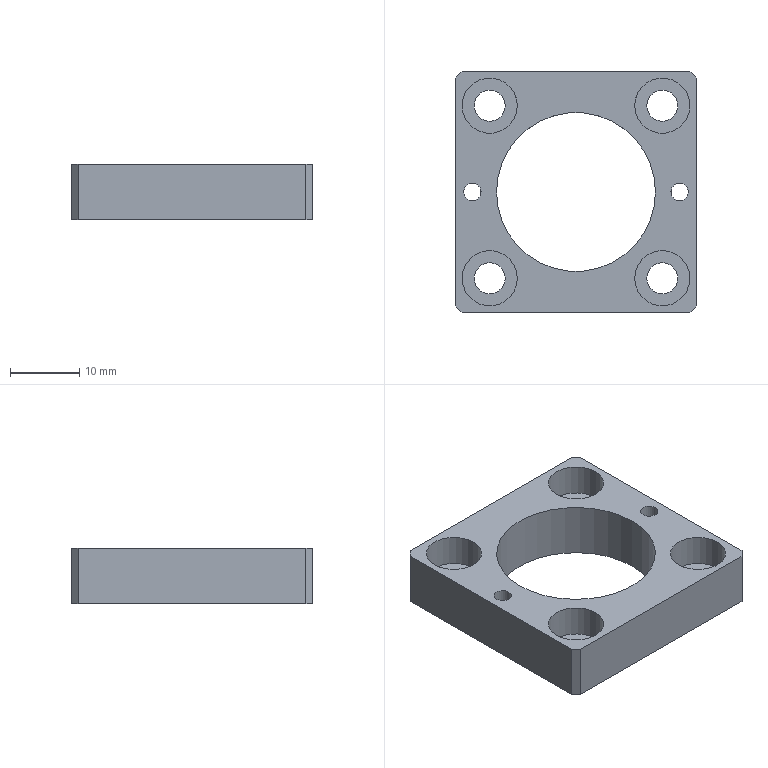Part | NX | 1 solid | 25 faces | box 35 x 35 x 8 mm | volume 5240 mm3 | plane 14 | cylinder 11 | commonest cylinder face diameters 4.5 x4 8 x4 2.5 x2 23 x1
STEP:
#1=CARTESIAN_POINT('',(14.75,-12.5,0.));
#2=VERTEX_POINT('',#1);
#3=CARTESIAN_POINT('',(12.5,-12.5,0.));
#4=DIRECTION('',(0.,0.,1.));
#5=DIRECTION('',(1.,0.,0.));
#6=AXIS2_PLACEMENT_3D('',#3,#4,#5);
#7=CIRCLE('',#6,2.25);
#8=EDGE_CURVE('',#2,#2,#7,.T.);
#9=ORIENTED_EDGE('',*,*,#8,.F.);
#10=EDGE_LOOP('',(#9));
#11=FACE_BOUND('',#10,.T.);
#12=CARTESIAN_POINT('',(14.75,-12.5,3.4));
#13=VERTEX_POINT('',#12);
#14=CARTESIAN_POINT('',(12.5,-12.5,3.4));
#15=DIRECTION('',(0.,0.,-1.));
#16=DIRECTION('',(1.,0.,0.));
#17=AXIS2_PLACEMENT_3D('',#14,#15,#16);
#18=CIRCLE('',#17,2.25);
#19=EDGE_CURVE('',#13,#13,#18,.T.);
#20=ORIENTED_EDGE('',*,*,#19,.F.);
#21=EDGE_LOOP('',(#20));
#22=FACE_BOUND('',#21,.T.);
#23=CARTESIAN_POINT('',(12.5,-12.5,0.));
#24=DIRECTION('',(0.,0.,1.));
#25=DIRECTION('',(-1.,0.,0.));
#26=AXIS2_PLACEMENT_3D('',#23,#24,#25);
#27=CYLINDRICAL_SURFACE('',#26,2.25);
#28=ADVANCED_FACE('',(#11,#22),#27,.F.);
#29=CARTESIAN_POINT('',(-10.25,-12.5,0.));
#30=VERTEX_POINT('',#29);
#31=CARTESIAN_POINT('',(-12.5,-12.5,0.));
#32=DIRECTION('',(0.,0.,1.));
#33=DIRECTION('',(1.,0.,0.));
#34=AXIS2_PLACEMENT_3D('',#31,#32,#33);
#35=CIRCLE('',#34,2.25);
#36=EDGE_CURVE('',#30,#30,#35,.T.);
#37=ORIENTED_EDGE('',*,*,#36,.F.);
#38=EDGE_LOOP('',(#37));
#39=FACE_BOUND('',#38,.T.);
#40=CARTESIAN_POINT('',(-10.25,-12.5,3.4));
#41=VERTEX_POINT('',#40);
#42=CARTESIAN_POINT('',(-12.5,-12.5,3.4));
#43=DIRECTION('',(0.,0.,-1.));
#44=DIRECTION('',(1.,0.,0.));
#45=AXIS2_PLACEMENT_3D('',#42,#43,#44);
#46=CIRCLE('',#45,2.25);
#47=EDGE_CURVE('',#41,#41,#46,.T.);
#48=ORIENTED_EDGE('',*,*,#47,.F.);
#49=EDGE_LOOP('',(#48));
#50=FACE_BOUND('',#49,.T.);
#51=CARTESIAN_POINT('',(-12.5,-12.5,0.));
#52=DIRECTION('',(0.,0.,1.));
#53=DIRECTION('',(-1.,0.,0.));
#54=AXIS2_PLACEMENT_3D('',#51,#52,#53);
#55=CYLINDRICAL_SURFACE('',#54,2.25);
#56=ADVANCED_FACE('',(#39,#50),#55,.F.);
#57=CARTESIAN_POINT('',(14.75,12.5,0.));
#58=VERTEX_POINT('',#57);
#59=CARTESIAN_POINT('',(12.5,12.5,0.));
#60=DIRECTION('',(0.,0.,1.));
#61=DIRECTION('',(1.,0.,0.));
#62=AXIS2_PLACEMENT_3D('',#59,#60,#61);
#63=CIRCLE('',#62,2.25);
#64=EDGE_CURVE('',#58,#58,#63,.T.);
#65=ORIENTED_EDGE('',*,*,#64,.F.);
#66=EDGE_LOOP('',(#65));
#67=FACE_BOUND('',#66,.T.);
#68=CARTESIAN_POINT('',(14.75,12.5,3.4));
#69=VERTEX_POINT('',#68);
#70=CARTESIAN_POINT('',(12.5,12.5,3.4));
#71=DIRECTION('',(0.,0.,-1.));
#72=DIRECTION('',(1.,0.,0.));
#73=AXIS2_PLACEMENT_3D('',#70,#71,#72);
#74=CIRCLE('',#73,2.25);
#75=EDGE_CURVE('',#69,#69,#74,.T.);
#76=ORIENTED_EDGE('',*,*,#75,.F.);
#77=EDGE_LOOP('',(#76));
#78=FACE_BOUND('',#77,.T.);
#79=CARTESIAN_POINT('',(12.5,12.5,0.));
#80=DIRECTION('',(0.,0.,1.));
#81=DIRECTION('',(-1.,0.,0.));
#82=AXIS2_PLACEMENT_3D('',#79,#80,#81);
#83=CYLINDRICAL_SURFACE('',#82,2.25);
#84=ADVANCED_FACE('',(#67,#78),#83,.F.);
#85=CARTESIAN_POINT('',(-13.75,0.,8.));
#86=VERTEX_POINT('',#85);
#87=CARTESIAN_POINT('',(-15.,0.,8.));
#88=DIRECTION('',(0.,0.,1.));
#89=DIRECTION('',(1.,0.,0.));
#90=AXIS2_PLACEMENT_3D('',#87,#88,#89);
#91=CIRCLE('',#90,1.25);
#92=EDGE_CURVE('',#86,#86,#91,.T.);
#93=ORIENTED_EDGE('',*,*,#92,.F.);
#94=EDGE_LOOP('',(#93));
#95=FACE_BOUND('',#94,.T.);
#96=CARTESIAN_POINT('',(11.5,0.,8.));
#97=VERTEX_POINT('',#96);
#98=CARTESIAN_POINT('',(0.,0.,8.));
#99=DIRECTION('',(0.,0.,1.));
#100=DIRECTION('',(1.,0.,0.));
#101=AXIS2_PLACEMENT_3D('',#98,#99,#100);
#102=CIRCLE('',#101,11.5);
#103=EDGE_CURVE('',#97,#97,#102,.T.);
#104=ORIENTED_EDGE('',*,*,#103,.F.);
#105=EDGE_LOOP('',(#104));
#106=FACE_BOUND('',#105,.T.);
#107=CARTESIAN_POINT('',(16.25,0.,8.));
#108=VERTEX_POINT('',#107);
#109=CARTESIAN_POINT('',(15.,0.,8.));
#110=DIRECTION('',(0.,0.,1.));
#111=DIRECTION('',(1.,0.,0.));
#112=AXIS2_PLACEMENT_3D('',#109,#110,#111);
#113=CIRCLE('',#112,1.25);
#114=EDGE_CURVE('',#108,#108,#113,.T.);
#115=ORIENTED_EDGE('',*,*,#114,.F.);
#116=EDGE_LOOP('',(#115));
#117=FACE_BOUND('',#116,.T.);
#118=CARTESIAN_POINT('',(-16.5,17.5,8.));
#119=VERTEX_POINT('',#118);
#120=CARTESIAN_POINT('',(16.5,17.5,8.));
#121=VERTEX_POINT('',#120);
#122=CARTESIAN_POINT('',(-16.5,17.5,8.));
#123=DIRECTION('',(1.,0.,0.));
#124=VECTOR('',#123,1.);
#125=LINE('',#122,#124);
#126=EDGE_CURVE('',#119,#121,#125,.T.);
#127=ORIENTED_EDGE('',*,*,#126,.F.);
#128=CARTESIAN_POINT('',(-17.5,16.5,8.));
#129=VERTEX_POINT('',#128);
#130=CARTESIAN_POINT('',(-17.5,16.5,8.));
#131=DIRECTION('',(0.7071,0.7071,0.));
#132=VECTOR('',#131,1.);
#133=LINE('',#130,#132);
#134=EDGE_CURVE('',#129,#119,#133,.T.);
#135=ORIENTED_EDGE('',*,*,#134,.F.);
#136=CARTESIAN_POINT('',(-17.5,-16.5,8.));
#137=VERTEX_POINT('',#136);
#138=CARTESIAN_POINT('',(-17.5,-16.5,8.));
#139=DIRECTION('',(0.,1.,0.));
#140=VECTOR('',#139,1.);
#141=LINE('',#138,#140);
#142=EDGE_CURVE('',#137,#129,#141,.T.);
#143=ORIENTED_EDGE('',*,*,#142,.F.);
#144=CARTESIAN_POINT('',(-16.5,-17.5,8.));
#145=VERTEX_POINT('',#144);
#146=CARTESIAN_POINT('',(-16.5,-17.5,8.));
#147=DIRECTION('',(-0.7071,0.7071,0.));
#148=VECTOR('',#147,1.);
#149=LINE('',#146,#148);
#150=EDGE_CURVE('',#145,#137,#149,.T.);
#151=ORIENTED_EDGE('',*,*,#150,.F.);
#152=CARTESIAN_POINT('',(16.5,-17.5,8.));
#153=VERTEX_POINT('',#152);
#154=CARTESIAN_POINT('',(16.5,-17.5,8.));
#155=DIRECTION('',(-1.,0.,0.));
#156=VECTOR('',#155,1.);
#157=LINE('',#154,#156);
#158=EDGE_CURVE('',#153,#145,#157,.T.);
#159=ORIENTED_EDGE('',*,*,#158,.F.);
#160=CARTESIAN_POINT('',(17.5,-16.5,8.));
#161=VERTEX_POINT('',#160);
#162=CARTESIAN_POINT('',(17.5,-16.5,8.));
#163=DIRECTION('',(-0.7071,-0.7071,0.));
#164=VECTOR('',#163,1.);
#165=LINE('',#162,#164);
#166=EDGE_CURVE('',#161,#153,#165,.T.);
#167=ORIENTED_EDGE('',*,*,#166,.F.);
#168=CARTESIAN_POINT('',(17.5,16.5,8.));
#169=VERTEX_POINT('',#168);
#170=CARTESIAN_POINT('',(17.5,16.5,8.));
#171=DIRECTION('',(0.,-1.,0.));
#172=VECTOR('',#171,1.);
#173=LINE('',#170,#172);
#174=EDGE_CURVE('',#169,#161,#173,.T.);
#175=ORIENTED_EDGE('',*,*,#174,.F.);
#176=CARTESIAN_POINT('',(16.5,17.5,8.));
#177=DIRECTION('',(0.7071,-0.7071,0.));
#178=VECTOR('',#177,1.);
#179=LINE('',#176,#178);
#180=EDGE_CURVE('',#121,#169,#179,.T.);
#181=ORIENTED_EDGE('',*,*,#180,.F.);
#182=EDGE_LOOP('',(#127,#135,#143,#151,#159,#167,#175,#181));
#183=FACE_BOUND('',#182,.T.);
#184=CARTESIAN_POINT('',(16.5,12.5,8.));
#185=VERTEX_POINT('',#184);
#186=CARTESIAN_POINT('',(12.5,12.5,8.));
#187=DIRECTION('',(0.,0.,1.));
#188=DIRECTION('',(1.,0.,0.));
#189=AXIS2_PLACEMENT_3D('',#186,#187,#188);
#190=CIRCLE('',#189,4.);
#191=EDGE_CURVE('',#185,#185,#190,.T.);
#192=ORIENTED_EDGE('',*,*,#191,.F.);
#193=EDGE_LOOP('',(#192));
#194=FACE_BOUND('',#193,.T.);
#195=CARTESIAN_POINT('',(16.5,-12.5,8.));
#196=VERTEX_POINT('',#195);
#197=CARTESIAN_POINT('',(12.5,-12.5,8.));
#198=DIRECTION('',(0.,0.,1.));
#199=DIRECTION('',(1.,0.,0.));
#200=AXIS2_PLACEMENT_3D('',#197,#198,#199);
#201=CIRCLE('',#200,4.);
#202=EDGE_CURVE('',#196,#196,#201,.T.);
#203=ORIENTED_EDGE('',*,*,#202,.F.);
#204=EDGE_LOOP('',(#203));
#205=FACE_BOUND('',#204,.T.);
#206=CARTESIAN_POINT('',(-8.5,-12.5,8.));
#207=VERTEX_POINT('',#206);
#208=CARTESIAN_POINT('',(-12.5,-12.5,8.));
#209=DIRECTION('',(0.,0.,1.));
#210=DIRECTION('',(1.,0.,0.));
#211=AXIS2_PLACEMENT_3D('',#208,#209,#210);
#212=CIRCLE('',#211,4.);
#213=EDGE_CURVE('',#207,#207,#212,.T.);
#214=ORIENTED_EDGE('',*,*,#213,.F.);
#215=EDGE_LOOP('',(#214));
#216=FACE_BOUND('',#215,.T.);
#217=CARTESIAN_POINT('',(-8.5,12.5,8.));
#218=VERTEX_POINT('',#217);
#219=CARTESIAN_POINT('',(-12.5,12.5,8.));
#220=DIRECTION('',(0.,0.,-1.));
#221=DIRECTION('',(1.,0.,0.));
#222=AXIS2_PLACEMENT_3D('',#219,#220,#221);
#223=CIRCLE('',#222,4.);
#224=EDGE_CURVE('',#218,#218,#223,.T.);
#225=ORIENTED_EDGE('',*,*,#224,.T.);
#226=EDGE_LOOP('',(#225));
#227=FACE_BOUND('',#226,.T.);
#228=CARTESIAN_POINT('',(15.,0.,8.));
#229=DIRECTION('',(0.,0.,1.));
#230=DIRECTION('',(-1.,0.,0.));
#231=AXIS2_PLACEMENT_3D('',#228,#229,#230);
#232=PLANE('',#231);
#233=ADVANCED_FACE('',(#95,#106,#117,#183,#194,#205,#216,#227),#232,.T.);
#234=ORIENTED_EDGE('',*,*,#126,.T.);
#235=CARTESIAN_POINT('',(16.5,17.5,0.));
#236=VERTEX_POINT('',#235);
#237=CARTESIAN_POINT('',(16.5,17.5,0.));
#238=DIRECTION('',(0.,0.,1.));
#239=VECTOR('',#238,1.);
#240=LINE('',#237,#239);
#241=EDGE_CURVE('',#236,#121,#240,.T.);
#242=ORIENTED_EDGE('',*,*,#241,.F.);
#243=CARTESIAN_POINT('',(-16.5,17.5,0.));
#244=VERTEX_POINT('',#243);
#245=CARTESIAN_POINT('',(-16.5,17.5,0.));
#246=DIRECTION('',(-1.,0.,0.));
#247=VECTOR('',#246,1.);
#248=LINE('',#245,#247);
#249=EDGE_CURVE('',#236,#244,#248,.T.);
#250=ORIENTED_EDGE('',*,*,#249,.T.);
#251=CARTESIAN_POINT('',(-16.5,17.5,0.));
#252=DIRECTION('',(0.,0.,1.));
#253=VECTOR('',#252,1.);
#254=LINE('',#251,#253);
#255=EDGE_CURVE('',#244,#119,#254,.T.);
#256=ORIENTED_EDGE('',*,*,#255,.T.);
#257=EDGE_LOOP('',(#234,#242,#250,#256));
#258=FACE_OUTER_BOUND('',#257,.T.);
#259=CARTESIAN_POINT('',(-16.5,17.5,0.));
#260=DIRECTION('',(0.,-1.,0.));
#261=DIRECTION('',(0.,0.,1.));
#262=AXIS2_PLACEMENT_3D('',#259,#260,#261);
#263=PLANE('',#262);
#264=ADVANCED_FACE('',(#258),#263,.F.);
#265=ORIENTED_EDGE('',*,*,#180,.T.);
#266=CARTESIAN_POINT('',(17.5,16.5,0.));
#267=VERTEX_POINT('',#266);
#268=CARTESIAN_POINT('',(17.5,16.5,0.));
#269=DIRECTION('',(0.,0.,1.));
#270=VECTOR('',#269,1.);
#271=LINE('',#268,#270);
#272=EDGE_CURVE('',#267,#169,#271,.T.);
#273=ORIENTED_EDGE('',*,*,#272,.F.);
#274=CARTESIAN_POINT('',(16.5,17.5,0.));
#275=DIRECTION('',(-0.7071,0.7071,0.));
#276=VECTOR('',#275,1.);
#277=LINE('',#274,#276);
#278=EDGE_CURVE('',#267,#236,#277,.T.);
#279=ORIENTED_EDGE('',*,*,#278,.T.);
#280=ORIENTED_EDGE('',*,*,#241,.T.);
#281=EDGE_LOOP('',(#265,#273,#279,#280));
#282=FACE_OUTER_BOUND('',#281,.T.);
#283=CARTESIAN_POINT('',(16.5,17.5,0.));
#284=DIRECTION('',(-0.7071,-0.7071,0.));
#285=DIRECTION('',(-0.7071,0.7071,0.));
#286=AXIS2_PLACEMENT_3D('',#283,#284,#285);
#287=PLANE('',#286);
#288=ADVANCED_FACE('',(#282),#287,.F.);
#289=ORIENTED_EDGE('',*,*,#174,.T.);
#290=CARTESIAN_POINT('',(17.5,-16.5,0.));
#291=VERTEX_POINT('',#290);
#292=CARTESIAN_POINT('',(17.5,-16.5,0.));
#293=DIRECTION('',(0.,0.,1.));
#294=VECTOR('',#293,1.);
#295=LINE('',#292,#294);
#296=EDGE_CURVE('',#291,#161,#295,.T.);
#297=ORIENTED_EDGE('',*,*,#296,.F.);
#298=CARTESIAN_POINT('',(17.5,16.5,0.));
#299=DIRECTION('',(0.,1.,0.));
#300=VECTOR('',#299,1.);
#301=LINE('',#298,#300);
#302=EDGE_CURVE('',#291,#267,#301,.T.);
#303=ORIENTED_EDGE('',*,*,#302,.T.);
#304=ORIENTED_EDGE('',*,*,#272,.T.);
#305=EDGE_LOOP('',(#289,#297,#303,#304));
#306=FACE_OUTER_BOUND('',#305,.T.);
#307=CARTESIAN_POINT('',(17.5,16.5,0.));
#308=DIRECTION('',(-1.,0.,0.));
#309=DIRECTION('',(0.,0.,-1.));
#310=AXIS2_PLACEMENT_3D('',#307,#308,#309);
#311=PLANE('',#310);
#312=ADVANCED_FACE('',(#306),#311,.F.);
#313=ORIENTED_EDGE('',*,*,#166,.T.);
#314=CARTESIAN_POINT('',(16.5,-17.5,0.));
#315=VERTEX_POINT('',#314);
#316=CARTESIAN_POINT('',(16.5,-17.5,0.));
#317=DIRECTION('',(0.,0.,1.));
#318=VECTOR('',#317,1.);
#319=LINE('',#316,#318);
#320=EDGE_CURVE('',#315,#153,#319,.T.);
#321=ORIENTED_EDGE('',*,*,#320,.F.);
#322=CARTESIAN_POINT('',(17.5,-16.5,0.));
#323=DIRECTION('',(0.7071,0.7071,0.));
#324=VECTOR('',#323,1.);
#325=LINE('',#322,#324);
#326=EDGE_CURVE('',#315,#291,#325,.T.);
#327=ORIENTED_EDGE('',*,*,#326,.T.);
#328=ORIENTED_EDGE('',*,*,#296,.T.);
#329=EDGE_LOOP('',(#313,#321,#327,#328));
#330=FACE_OUTER_BOUND('',#329,.T.);
#331=CARTESIAN_POINT('',(17.5,-16.5,0.));
#332=DIRECTION('',(-0.7071,0.7071,0.));
#333=DIRECTION('',(0.7071,0.7071,0.));
#334=AXIS2_PLACEMENT_3D('',#331,#332,#333);
#335=PLANE('',#334);
#336=ADVANCED_FACE('',(#330),#335,.F.);
#337=ORIENTED_EDGE('',*,*,#158,.T.);
#338=CARTESIAN_POINT('',(-16.5,-17.5,0.));
#339=VERTEX_POINT('',#338);
#340=CARTESIAN_POINT('',(-16.5,-17.5,0.));
#341=DIRECTION('',(0.,0.,1.));
#342=VECTOR('',#341,1.);
#343=LINE('',#340,#342);
#344=EDGE_CURVE('',#339,#145,#343,.T.);
#345=ORIENTED_EDGE('',*,*,#344,.F.);
#346=CARTESIAN_POINT('',(16.5,-17.5,0.));
#347=DIRECTION('',(1.,0.,0.));
#348=VECTOR('',#347,1.);
#349=LINE('',#346,#348);
#350=EDGE_CURVE('',#339,#315,#349,.T.);
#351=ORIENTED_EDGE('',*,*,#350,.T.);
#352=ORIENTED_EDGE('',*,*,#320,.T.);
#353=EDGE_LOOP('',(#337,#345,#351,#352));
#354=FACE_OUTER_BOUND('',#353,.T.);
#355=CARTESIAN_POINT('',(16.5,-17.5,0.));
#356=DIRECTION('',(0.,1.,0.));
#357=DIRECTION('',(0.,0.,-1.));
#358=AXIS2_PLACEMENT_3D('',#355,#356,#357);
#359=PLANE('',#358);
#360=ADVANCED_FACE('',(#354),#359,.F.);
#361=ORIENTED_EDGE('',*,*,#150,.T.);
#362=CARTESIAN_POINT('',(-17.5,-16.5,0.));
#363=VERTEX_POINT('',#362);
#364=CARTESIAN_POINT('',(-17.5,-16.5,0.));
#365=DIRECTION('',(0.,0.,1.));
#366=VECTOR('',#365,1.);
#367=LINE('',#364,#366);
#368=EDGE_CURVE('',#363,#137,#367,.T.);
#369=ORIENTED_EDGE('',*,*,#368,.F.);
#370=CARTESIAN_POINT('',(-16.5,-17.5,0.));
#371=DIRECTION('',(0.7071,-0.7071,0.));
#372=VECTOR('',#371,1.);
#373=LINE('',#370,#372);
#374=EDGE_CURVE('',#363,#339,#373,.T.);
#375=ORIENTED_EDGE('',*,*,#374,.T.);
#376=ORIENTED_EDGE('',*,*,#344,.T.);
#377=EDGE_LOOP('',(#361,#369,#375,#376));
#378=FACE_OUTER_BOUND('',#377,.T.);
#379=CARTESIAN_POINT('',(-16.5,-17.5,0.));
#380=DIRECTION('',(0.7071,0.7071,0.));
#381=DIRECTION('',(0.7071,-0.7071,0.));
#382=AXIS2_PLACEMENT_3D('',#379,#380,#381);
#383=PLANE('',#382);
#384=ADVANCED_FACE('',(#378),#383,.F.);
#385=ORIENTED_EDGE('',*,*,#142,.T.);
#386=CARTESIAN_POINT('',(-17.5,16.5,0.));
#387=VERTEX_POINT('',#386);
#388=CARTESIAN_POINT('',(-17.5,16.5,0.));
#389=DIRECTION('',(0.,0.,1.));
#390=VECTOR('',#389,1.);
#391=LINE('',#388,#390);
#392=EDGE_CURVE('',#387,#129,#391,.T.);
#393=ORIENTED_EDGE('',*,*,#392,.F.);
#394=CARTESIAN_POINT('',(-17.5,-16.5,0.));
#395=DIRECTION('',(0.,-1.,0.));
#396=VECTOR('',#395,1.);
#397=LINE('',#394,#396);
#398=EDGE_CURVE('',#387,#363,#397,.T.);
#399=ORIENTED_EDGE('',*,*,#398,.T.);
#400=ORIENTED_EDGE('',*,*,#368,.T.);
#401=EDGE_LOOP('',(#385,#393,#399,#400));
#402=FACE_OUTER_BOUND('',#401,.T.);
#403=CARTESIAN_POINT('',(-17.5,-16.5,0.));
#404=DIRECTION('',(1.,0.,0.));
#405=DIRECTION('',(0.,0.,1.));
#406=AXIS2_PLACEMENT_3D('',#403,#404,#405);
#407=PLANE('',#406);
#408=ADVANCED_FACE('',(#402),#407,.F.);
#409=ORIENTED_EDGE('',*,*,#92,.T.);
#410=EDGE_LOOP('',(#409));
#411=FACE_BOUND('',#410,.T.);
#412=CARTESIAN_POINT('',(-13.75,0.,0.));
#413=VERTEX_POINT('',#412);
#414=CARTESIAN_POINT('',(-15.,0.,0.));
#415=DIRECTION('',(0.,0.,-1.));
#416=DIRECTION('',(1.,0.,0.));
#417=AXIS2_PLACEMENT_3D('',#414,#415,#416);
#418=CIRCLE('',#417,1.25);
#419=EDGE_CURVE('',#413,#413,#418,.T.);
#420=ORIENTED_EDGE('',*,*,#419,.T.);
#421=EDGE_LOOP('',(#420));
#422=FACE_BOUND('',#421,.T.);
#423=CARTESIAN_POINT('',(-15.,0.,0.));
#424=DIRECTION('',(0.,0.,1.));
#425=DIRECTION('',(-1.,0.,0.));
#426=AXIS2_PLACEMENT_3D('',#423,#424,#425);
#427=CYLINDRICAL_SURFACE('',#426,1.25);
#428=ADVANCED_FACE('',(#411,#422),#427,.F.);
#429=CARTESIAN_POINT('',(-14.75,12.5,3.4));
#430=VERTEX_POINT('',#429);
#431=CARTESIAN_POINT('',(-12.5,12.5,3.4));
#432=DIRECTION('',(0.,0.,1.));
#433=DIRECTION('',(-1.,0.,0.));
#434=AXIS2_PLACEMENT_3D('',#431,#432,#433);
#435=CIRCLE('',#434,2.25);
#436=EDGE_CURVE('',#430,#430,#435,.T.);
#437=ORIENTED_EDGE('',*,*,#436,.T.);
#438=EDGE_LOOP('',(#437));
#439=FACE_BOUND('',#438,.T.);
#440=CARTESIAN_POINT('',(-10.25,12.5,0.));
#441=VERTEX_POINT('',#440);
#442=CARTESIAN_POINT('',(-12.5,12.5,0.));
#443=DIRECTION('',(0.,0.,-1.));
#444=DIRECTION('',(1.,0.,0.));
#445=AXIS2_PLACEMENT_3D('',#442,#443,#444);
#446=CIRCLE('',#445,2.25);
#447=EDGE_CURVE('',#441,#441,#446,.T.);
#448=ORIENTED_EDGE('',*,*,#447,.T.);
#449=EDGE_LOOP('',(#448));
#450=FACE_BOUND('',#449,.T.);
#451=CARTESIAN_POINT('',(-12.5,12.5,0.));
#452=DIRECTION('',(0.,0.,1.));
#453=DIRECTION('',(-1.,0.,0.));
#454=AXIS2_PLACEMENT_3D('',#451,#452,#453);
#455=CYLINDRICAL_SURFACE('',#454,2.25);
#456=ADVANCED_FACE('',(#439,#450),#455,.F.);
#457=ORIENTED_EDGE('',*,*,#103,.T.);
#458=EDGE_LOOP('',(#457));
#459=FACE_BOUND('',#458,.T.);
#460=CARTESIAN_POINT('',(11.5,0.,0.));
#461=VERTEX_POINT('',#460);
#462=CARTESIAN_POINT('',(0.,0.,0.));
#463=DIRECTION('',(0.,0.,-1.));
#464=DIRECTION('',(1.,0.,0.));
#465=AXIS2_PLACEMENT_3D('',#462,#463,#464);
#466=CIRCLE('',#465,11.5);
#467=EDGE_CURVE('',#461,#461,#466,.T.);
#468=ORIENTED_EDGE('',*,*,#467,.T.);
#469=EDGE_LOOP('',(#468));
#470=FACE_BOUND('',#469,.T.);
#471=CARTESIAN_POINT('',(0.,0.,0.));
#472=DIRECTION('',(0.,0.,1.));
#473=DIRECTION('',(-1.,0.,0.));
#474=AXIS2_PLACEMENT_3D('',#471,#472,#473);
#475=CYLINDRICAL_SURFACE('',#474,11.5);
#476=ADVANCED_FACE('',(#459,#470),#475,.F.);
#477=ORIENTED_EDGE('',*,*,#114,.T.);
#478=EDGE_LOOP('',(#477));
#479=FACE_BOUND('',#478,.T.);
#480=CARTESIAN_POINT('',(16.25,0.,0.));
#481=VERTEX_POINT('',#480);
#482=CARTESIAN_POINT('',(15.,0.,0.));
#483=DIRECTION('',(0.,0.,-1.));
#484=DIRECTION('',(1.,0.,0.));
#485=AXIS2_PLACEMENT_3D('',#482,#483,#484);
#486=CIRCLE('',#485,1.25);
#487=EDGE_CURVE('',#481,#481,#486,.T.);
#488=ORIENTED_EDGE('',*,*,#487,.T.);
#489=EDGE_LOOP('',(#488));
#490=FACE_BOUND('',#489,.T.);
#491=CARTESIAN_POINT('',(15.,0.,0.));
#492=DIRECTION('',(0.,0.,1.));
#493=DIRECTION('',(-1.,0.,0.));
#494=AXIS2_PLACEMENT_3D('',#491,#492,#493);
#495=CYLINDRICAL_SURFACE('',#494,1.25);
#496=ADVANCED_FACE('',(#479,#490),#495,.F.);
#497=ORIENTED_EDGE('',*,*,#134,.T.);
#498=ORIENTED_EDGE('',*,*,#255,.F.);
#499=CARTESIAN_POINT('',(-17.5,16.5,0.));
#500=DIRECTION('',(-0.7071,-0.7071,0.));
#501=VECTOR('',#500,1.);
#502=LINE('',#499,#501);
#503=EDGE_CURVE('',#244,#387,#502,.T.);
#504=ORIENTED_EDGE('',*,*,#503,.T.);
#505=ORIENTED_EDGE('',*,*,#392,.T.);
#506=EDGE_LOOP('',(#497,#498,#504,#505));
#507=FACE_OUTER_BOUND('',#506,.T.);
#508=CARTESIAN_POINT('',(-17.5,16.5,0.));
#509=DIRECTION('',(0.7071,-0.7071,0.));
#510=DIRECTION('',(-0.7071,-0.7071,0.));
#511=AXIS2_PLACEMENT_3D('',#508,#509,#510);
#512=PLANE('',#511);
#513=ADVANCED_FACE('',(#507),#512,.F.);
#514=ORIENTED_EDGE('',*,*,#249,.F.);
#515=ORIENTED_EDGE('',*,*,#278,.F.);
#516=ORIENTED_EDGE('',*,*,#302,.F.);
#517=ORIENTED_EDGE('',*,*,#326,.F.);
#518=ORIENTED_EDGE('',*,*,#350,.F.);
#519=ORIENTED_EDGE('',*,*,#374,.F.);
#520=ORIENTED_EDGE('',*,*,#398,.F.);
#521=ORIENTED_EDGE('',*,*,#503,.F.);
#522=EDGE_LOOP('',(#514,#515,#516,#517,#518,#519,#520,#521));
#523=FACE_BOUND('',#522,.T.);
#524=ORIENTED_EDGE('',*,*,#487,.F.);
#525=EDGE_LOOP('',(#524));
#526=FACE_BOUND('',#525,.T.);
#527=ORIENTED_EDGE('',*,*,#467,.F.);
#528=EDGE_LOOP('',(#527));
#529=FACE_BOUND('',#528,.T.);
#530=ORIENTED_EDGE('',*,*,#447,.F.);
#531=EDGE_LOOP('',(#530));
#532=FACE_BOUND('',#531,.T.);
#533=ORIENTED_EDGE('',*,*,#419,.F.);
#534=EDGE_LOOP('',(#533));
#535=FACE_BOUND('',#534,.T.);
#536=ORIENTED_EDGE('',*,*,#36,.T.);
#537=EDGE_LOOP('',(#536));
#538=FACE_BOUND('',#537,.T.);
#539=ORIENTED_EDGE('',*,*,#8,.T.);
#540=EDGE_LOOP('',(#539));
#541=FACE_BOUND('',#540,.T.);
#542=ORIENTED_EDGE('',*,*,#64,.T.);
#543=EDGE_LOOP('',(#542));
#544=FACE_BOUND('',#543,.T.);
#545=CARTESIAN_POINT('',(15.,0.,0.));
#546=DIRECTION('',(0.,0.,1.));
#547=DIRECTION('',(-1.,0.,0.));
#548=AXIS2_PLACEMENT_3D('',#545,#546,#547);
#549=PLANE('',#548);
#550=ADVANCED_FACE('',(#523,#526,#529,#532,#535,#538,#541,#544),#549,.F.);
#551=ORIENTED_EDGE('',*,*,#191,.T.);
#552=EDGE_LOOP('',(#551));
#553=FACE_BOUND('',#552,.T.);
#554=CARTESIAN_POINT('',(16.5,12.5,3.4));
#555=VERTEX_POINT('',#554);
#556=CARTESIAN_POINT('',(12.5,12.5,3.4));
#557=DIRECTION('',(0.,0.,-1.));
#558=DIRECTION('',(1.,0.,0.));
#559=AXIS2_PLACEMENT_3D('',#556,#557,#558);
#560=CIRCLE('',#559,4.);
#561=EDGE_CURVE('',#555,#555,#560,.T.);
#562=ORIENTED_EDGE('',*,*,#561,.T.);
#563=EDGE_LOOP('',(#562));
#564=FACE_BOUND('',#563,.T.);
#565=CARTESIAN_POINT('',(12.5,12.5,3.4));
#566=DIRECTION('',(0.,0.,1.));
#567=DIRECTION('',(-1.,0.,0.));
#568=AXIS2_PLACEMENT_3D('',#565,#566,#567);
#569=CYLINDRICAL_SURFACE('',#568,4.);
#570=ADVANCED_FACE('',(#553,#564),#569,.F.);
#571=ORIENTED_EDGE('',*,*,#75,.T.);
#572=EDGE_LOOP('',(#571));
#573=FACE_BOUND('',#572,.T.);
#574=ORIENTED_EDGE('',*,*,#561,.F.);
#575=EDGE_LOOP('',(#574));
#576=FACE_BOUND('',#575,.T.);
#577=CARTESIAN_POINT('',(12.5,12.5,3.4));
#578=DIRECTION('',(0.,0.,1.));
#579=DIRECTION('',(-1.,0.,0.));
#580=AXIS2_PLACEMENT_3D('',#577,#578,#579);
#581=PLANE('',#580);
#582=ADVANCED_FACE('',(#573,#576),#581,.T.);
#583=ORIENTED_EDGE('',*,*,#202,.T.);
#584=EDGE_LOOP('',(#583));
#585=FACE_BOUND('',#584,.T.);
#586=CARTESIAN_POINT('',(16.5,-12.5,3.4));
#587=VERTEX_POINT('',#586);
#588=CARTESIAN_POINT('',(12.5,-12.5,3.4));
#589=DIRECTION('',(0.,0.,-1.));
#590=DIRECTION('',(1.,0.,0.));
#591=AXIS2_PLACEMENT_3D('',#588,#589,#590);
#592=CIRCLE('',#591,4.);
#593=EDGE_CURVE('',#587,#587,#592,.T.);
#594=ORIENTED_EDGE('',*,*,#593,.T.);
#595=EDGE_LOOP('',(#594));
#596=FACE_BOUND('',#595,.T.);
#597=CARTESIAN_POINT('',(12.5,-12.5,3.4));
#598=DIRECTION('',(0.,0.,1.));
#599=DIRECTION('',(-1.,0.,0.));
#600=AXIS2_PLACEMENT_3D('',#597,#598,#599);
#601=CYLINDRICAL_SURFACE('',#600,4.);
#602=ADVANCED_FACE('',(#585,#596),#601,.F.);
#603=ORIENTED_EDGE('',*,*,#19,.T.);
#604=EDGE_LOOP('',(#603));
#605=FACE_BOUND('',#604,.T.);
#606=ORIENTED_EDGE('',*,*,#593,.F.);
#607=EDGE_LOOP('',(#606));
#608=FACE_BOUND('',#607,.T.);
#609=CARTESIAN_POINT('',(12.5,-12.5,3.4));
#610=DIRECTION('',(0.,0.,1.));
#611=DIRECTION('',(-1.,0.,0.));
#612=AXIS2_PLACEMENT_3D('',#609,#610,#611);
#613=PLANE('',#612);
#614=ADVANCED_FACE('',(#605,#608),#613,.T.);
#615=ORIENTED_EDGE('',*,*,#213,.T.);
#616=EDGE_LOOP('',(#615));
#617=FACE_BOUND('',#616,.T.);
#618=CARTESIAN_POINT('',(-8.5,-12.5,3.4));
#619=VERTEX_POINT('',#618);
#620=CARTESIAN_POINT('',(-12.5,-12.5,3.4));
#621=DIRECTION('',(0.,0.,-1.));
#622=DIRECTION('',(1.,0.,0.));
#623=AXIS2_PLACEMENT_3D('',#620,#621,#622);
#624=CIRCLE('',#623,4.);
#625=EDGE_CURVE('',#619,#619,#624,.T.);
#626=ORIENTED_EDGE('',*,*,#625,.T.);
#627=EDGE_LOOP('',(#626));
#628=FACE_BOUND('',#627,.T.);
#629=CARTESIAN_POINT('',(-12.5,-12.5,3.4));
#630=DIRECTION('',(0.,0.,1.));
#631=DIRECTION('',(-1.,0.,0.));
#632=AXIS2_PLACEMENT_3D('',#629,#630,#631);
#633=CYLINDRICAL_SURFACE('',#632,4.);
#634=ADVANCED_FACE('',(#617,#628),#633,.F.);
#635=ORIENTED_EDGE('',*,*,#47,.T.);
#636=EDGE_LOOP('',(#635));
#637=FACE_BOUND('',#636,.T.);
#638=ORIENTED_EDGE('',*,*,#625,.F.);
#639=EDGE_LOOP('',(#638));
#640=FACE_BOUND('',#639,.T.);
#641=CARTESIAN_POINT('',(-12.5,-12.5,3.4));
#642=DIRECTION('',(0.,0.,1.));
#643=DIRECTION('',(-1.,0.,0.));
#644=AXIS2_PLACEMENT_3D('',#641,#642,#643);
#645=PLANE('',#644);
#646=ADVANCED_FACE('',(#637,#640),#645,.T.);
#647=CARTESIAN_POINT('',(-8.5,12.5,3.4));
#648=VERTEX_POINT('',#647);
#649=CARTESIAN_POINT('',(-12.5,12.5,3.4));
#650=DIRECTION('',(0.,0.,1.));
#651=DIRECTION('',(1.,0.,0.));
#652=AXIS2_PLACEMENT_3D('',#649,#650,#651);
#653=CIRCLE('',#652,4.);
#654=EDGE_CURVE('',#648,#648,#653,.T.);
#655=ORIENTED_EDGE('',*,*,#654,.T.);
#656=EDGE_LOOP('',(#655));
#657=FACE_BOUND('',#656,.T.);
#658=ORIENTED_EDGE('',*,*,#436,.F.);
#659=EDGE_LOOP('',(#658));
#660=FACE_BOUND('',#659,.T.);
#661=CARTESIAN_POINT('',(-12.5,12.5,3.4));
#662=DIRECTION('',(0.,0.,-1.));
#663=DIRECTION('',(1.,0.,0.));
#664=AXIS2_PLACEMENT_3D('',#661,#662,#663);
#665=PLANE('',#664);
#666=ADVANCED_FACE('',(#657,#660),#665,.F.);
#667=ORIENTED_EDGE('',*,*,#224,.F.);
#668=EDGE_LOOP('',(#667));
#669=FACE_BOUND('',#668,.T.);
#670=ORIENTED_EDGE('',*,*,#654,.F.);
#671=EDGE_LOOP('',(#670));
#672=FACE_BOUND('',#671,.T.);
#673=CARTESIAN_POINT('',(-12.5,12.5,3.4));
#674=DIRECTION('',(0.,0.,1.));
#675=DIRECTION('',(-1.,0.,0.));
#676=AXIS2_PLACEMENT_3D('',#673,#674,#675);
#677=CYLINDRICAL_SURFACE('',#676,4.);
#678=ADVANCED_FACE('',(#669,#672),#677,.F.);
#679=CLOSED_SHELL('',(#28,#56,#84,#233,#264,#288,#312,#336,#360,#384,#408,#428,#456,#476,#496,#513,#550,#570,#582,#602,#614,#634,#646,#666,#678));
#680=MANIFOLD_SOLID_BREP('',#679);
#681=(LENGTH_UNIT()NAMED_UNIT(*)SI_UNIT(.MILLI.,.METRE.));
#682=UNCERTAINTY_MEASURE_WITH_UNIT(LENGTH_MEASURE(0.00002),#681,'','');
#683=(NAMED_UNIT(*)PLANE_ANGLE_UNIT()SI_UNIT($,.RADIAN.));
#684=PLANE_ANGLE_MEASURE_WITH_UNIT(PLANE_ANGLE_MEASURE(0.01745),#683);
#685=DIMENSIONAL_EXPONENTS(0.,0.,0.,0.,0.,0.,0.);
#686=(CONVERSION_BASED_UNIT('DEGREE',#684)NAMED_UNIT(#685)PLANE_ANGLE_UNIT());
#687=(NAMED_UNIT(*)SI_UNIT($,.STERADIAN.)SOLID_ANGLE_UNIT());
#688=(GEOMETRIC_REPRESENTATION_CONTEXT(3)GLOBAL_UNCERTAINTY_ASSIGNED_CONTEXT((#682))GLOBAL_UNIT_ASSIGNED_CONTEXT((#681,#686,#687))REPRESENTATION_CONTEXT('',''));
#689=ADVANCED_BREP_SHAPE_REPRESENTATION('',(#680),#688);